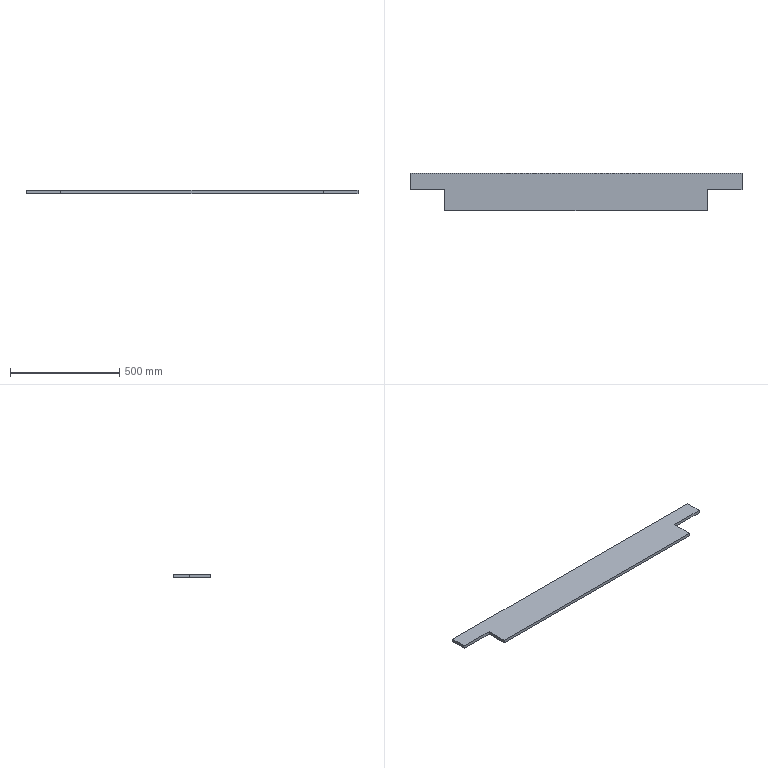Part | SolidWorks | features BaseBody 1 | 1 solid | 10 faces | box 1520 x 172 x 14 mm | volume 3225600 mm3 | plane 10
STEP:
#1=CARTESIAN_POINT('',(-600.,-84.5,14.));
#2=VERTEX_POINT('',#1);
#3=CARTESIAN_POINT('',(-600.,12.5,14.));
#4=VERTEX_POINT('',#3);
#5=CARTESIAN_POINT('',(-600.,12.5,14.));
#6=DIRECTION('',(0.,1.,0.));
#7=VECTOR('',#6,1000.);
#8=LINE('',#5,#7);
#9=EDGE_CURVE('',#2,#4,#8,.T.);
#10=ORIENTED_EDGE('',*,*,#9,.F.);
#11=CARTESIAN_POINT('',(600.,-84.5,14.));
#12=VERTEX_POINT('',#11);
#13=CARTESIAN_POINT('',(-600.,-84.5,14.));
#14=DIRECTION('',(-1.,0.,0.));
#15=VECTOR('',#14,1000.);
#16=LINE('',#13,#15);
#17=EDGE_CURVE('',#12,#2,#16,.T.);
#18=ORIENTED_EDGE('',*,*,#17,.F.);
#19=CARTESIAN_POINT('',(600.,12.5,14.));
#20=VERTEX_POINT('',#19);
#21=CARTESIAN_POINT('',(600.,12.5,14.));
#22=DIRECTION('',(0.,-1.,0.));
#23=VECTOR('',#22,1000.);
#24=LINE('',#21,#23);
#25=EDGE_CURVE('',#20,#12,#24,.T.);
#26=ORIENTED_EDGE('',*,*,#25,.F.);
#27=CARTESIAN_POINT('',(760.,12.5,14.));
#28=VERTEX_POINT('',#27);
#29=CARTESIAN_POINT('',(760.,12.5,14.));
#30=DIRECTION('',(-1.,0.,0.));
#31=VECTOR('',#30,1000.);
#32=LINE('',#29,#31);
#33=EDGE_CURVE('',#28,#20,#32,.T.);
#34=ORIENTED_EDGE('',*,*,#33,.F.);
#35=CARTESIAN_POINT('',(760.,87.5,14.));
#36=VERTEX_POINT('',#35);
#37=CARTESIAN_POINT('',(760.,87.5,14.));
#38=DIRECTION('',(0.,1.,0.));
#39=VECTOR('',#38,1000.);
#40=LINE('',#37,#39);
#41=EDGE_CURVE('',#28,#36,#40,.T.);
#42=ORIENTED_EDGE('',*,*,#41,.T.);
#43=CARTESIAN_POINT('',(-760.,87.5,14.));
#44=VERTEX_POINT('',#43);
#45=CARTESIAN_POINT('',(-760.,87.5,14.));
#46=DIRECTION('',(-1.,0.,0.));
#47=VECTOR('',#46,1000.);
#48=LINE('',#45,#47);
#49=EDGE_CURVE('',#36,#44,#48,.T.);
#50=ORIENTED_EDGE('',*,*,#49,.T.);
#51=CARTESIAN_POINT('',(-760.,12.5,14.));
#52=VERTEX_POINT('',#51);
#53=CARTESIAN_POINT('',(-760.,87.5,14.));
#54=DIRECTION('',(0.,-1.,0.));
#55=VECTOR('',#54,1000.);
#56=LINE('',#53,#55);
#57=EDGE_CURVE('',#44,#52,#56,.T.);
#58=ORIENTED_EDGE('',*,*,#57,.T.);
#59=CARTESIAN_POINT('',(-760.,12.5,14.));
#60=DIRECTION('',(-1.,0.,0.));
#61=VECTOR('',#60,1000.);
#62=LINE('',#59,#61);
#63=EDGE_CURVE('',#4,#52,#62,.T.);
#64=ORIENTED_EDGE('',*,*,#63,.F.);
#65=EDGE_LOOP('',(#10,#18,#26,#34,#42,#50,#58,#64));
#66=FACE_OUTER_BOUND('',#65,.T.);
#67=CARTESIAN_POINT('',(0.,0.,14.));
#68=DIRECTION('',(0.,0.,1.));
#69=DIRECTION('',(1.,0.,0.));
#70=AXIS2_PLACEMENT_3D('',#67,#68,#69);
#71=PLANE('',#70);
#72=ADVANCED_FACE('',(#66),#71,.T.);
#73=CARTESIAN_POINT('',(-600.,-84.5,0.));
#74=VERTEX_POINT('',#73);
#75=CARTESIAN_POINT('',(600.,-84.5,0.));
#76=VERTEX_POINT('',#75);
#77=CARTESIAN_POINT('',(0.,-84.5,0.));
#78=DIRECTION('',(1.,0.,0.));
#79=VECTOR('',#78,1000.);
#80=LINE('',#77,#79);
#81=EDGE_CURVE('',#74,#76,#80,.T.);
#82=ORIENTED_EDGE('',*,*,#81,.F.);
#83=CARTESIAN_POINT('',(-600.,12.5,0.));
#84=VERTEX_POINT('',#83);
#85=CARTESIAN_POINT('',(-600.,12.5,0.));
#86=DIRECTION('',(0.,1.,0.));
#87=VECTOR('',#86,1000.);
#88=LINE('',#85,#87);
#89=EDGE_CURVE('',#74,#84,#88,.T.);
#90=ORIENTED_EDGE('',*,*,#89,.T.);
#91=CARTESIAN_POINT('',(-760.,12.5,0.));
#92=VERTEX_POINT('',#91);
#93=CARTESIAN_POINT('',(-760.,12.5,0.));
#94=DIRECTION('',(-1.,0.,0.));
#95=VECTOR('',#94,1000.);
#96=LINE('',#93,#95);
#97=EDGE_CURVE('',#84,#92,#96,.T.);
#98=ORIENTED_EDGE('',*,*,#97,.T.);
#99=CARTESIAN_POINT('',(-760.,87.5,0.));
#100=VERTEX_POINT('',#99);
#101=CARTESIAN_POINT('',(-760.,87.5,0.));
#102=DIRECTION('',(0.,-1.,0.));
#103=VECTOR('',#102,1000.);
#104=LINE('',#101,#103);
#105=EDGE_CURVE('',#100,#92,#104,.T.);
#106=ORIENTED_EDGE('',*,*,#105,.F.);
#107=CARTESIAN_POINT('',(760.,87.5,0.));
#108=VERTEX_POINT('',#107);
#109=CARTESIAN_POINT('',(-760.,87.5,0.));
#110=DIRECTION('',(-1.,0.,0.));
#111=VECTOR('',#110,1000.);
#112=LINE('',#109,#111);
#113=EDGE_CURVE('',#108,#100,#112,.T.);
#114=ORIENTED_EDGE('',*,*,#113,.F.);
#115=CARTESIAN_POINT('',(760.,12.5,0.));
#116=VERTEX_POINT('',#115);
#117=CARTESIAN_POINT('',(760.,87.5,0.));
#118=DIRECTION('',(0.,1.,0.));
#119=VECTOR('',#118,1000.);
#120=LINE('',#117,#119);
#121=EDGE_CURVE('',#116,#108,#120,.T.);
#122=ORIENTED_EDGE('',*,*,#121,.F.);
#123=CARTESIAN_POINT('',(600.,12.5,0.));
#124=VERTEX_POINT('',#123);
#125=CARTESIAN_POINT('',(760.,12.5,0.));
#126=DIRECTION('',(-1.,0.,0.));
#127=VECTOR('',#126,1000.);
#128=LINE('',#125,#127);
#129=EDGE_CURVE('',#116,#124,#128,.T.);
#130=ORIENTED_EDGE('',*,*,#129,.T.);
#131=CARTESIAN_POINT('',(600.,12.5,0.));
#132=DIRECTION('',(0.,-1.,0.));
#133=VECTOR('',#132,1000.);
#134=LINE('',#131,#133);
#135=EDGE_CURVE('',#124,#76,#134,.T.);
#136=ORIENTED_EDGE('',*,*,#135,.T.);
#137=EDGE_LOOP('',(#82,#90,#98,#106,#114,#122,#130,#136));
#138=FACE_OUTER_BOUND('',#137,.T.);
#139=CARTESIAN_POINT('',(0.,0.,0.));
#140=DIRECTION('',(0.,0.,1.));
#141=DIRECTION('',(1.,0.,0.));
#142=AXIS2_PLACEMENT_3D('',#139,#140,#141);
#143=PLANE('',#142);
#144=ADVANCED_FACE('',(#138),#143,.F.);
#145=CARTESIAN_POINT('',(600.,-84.5,14.));
#146=DIRECTION('',(0.,0.,1.));
#147=VECTOR('',#146,1000.);
#148=LINE('',#145,#147);
#149=EDGE_CURVE('',#76,#12,#148,.T.);
#150=ORIENTED_EDGE('',*,*,#149,.F.);
#151=ORIENTED_EDGE('',*,*,#135,.F.);
#152=CARTESIAN_POINT('',(600.,12.5,0.));
#153=DIRECTION('',(0.,0.,1.));
#154=VECTOR('',#153,1000.);
#155=LINE('',#152,#154);
#156=EDGE_CURVE('',#124,#20,#155,.T.);
#157=ORIENTED_EDGE('',*,*,#156,.T.);
#158=ORIENTED_EDGE('',*,*,#25,.T.);
#159=EDGE_LOOP('',(#150,#151,#157,#158));
#160=FACE_OUTER_BOUND('',#159,.T.);
#161=CARTESIAN_POINT('',(600.,12.5,0.));
#162=DIRECTION('',(-1.,0.,0.));
#163=DIRECTION('',(0.,0.,1.));
#164=AXIS2_PLACEMENT_3D('',#161,#162,#163);
#165=PLANE('',#164);
#166=ADVANCED_FACE('',(#160),#165,.F.);
#167=CARTESIAN_POINT('',(-600.,-84.5,14.));
#168=DIRECTION('',(0.,0.,-1.));
#169=VECTOR('',#168,1000.);
#170=LINE('',#167,#169);
#171=EDGE_CURVE('',#2,#74,#170,.T.);
#172=ORIENTED_EDGE('',*,*,#171,.F.);
#173=ORIENTED_EDGE('',*,*,#9,.T.);
#174=CARTESIAN_POINT('',(-600.,12.5,0.));
#175=DIRECTION('',(0.,0.,1.));
#176=VECTOR('',#175,1000.);
#177=LINE('',#174,#176);
#178=EDGE_CURVE('',#84,#4,#177,.T.);
#179=ORIENTED_EDGE('',*,*,#178,.F.);
#180=ORIENTED_EDGE('',*,*,#89,.F.);
#181=EDGE_LOOP('',(#172,#173,#179,#180));
#182=FACE_OUTER_BOUND('',#181,.T.);
#183=CARTESIAN_POINT('',(-600.,12.5,0.));
#184=DIRECTION('',(1.,0.,0.));
#185=DIRECTION('',(0.,0.,-1.));
#186=AXIS2_PLACEMENT_3D('',#183,#184,#185);
#187=PLANE('',#186);
#188=ADVANCED_FACE('',(#182),#187,.F.);
#189=ORIENTED_EDGE('',*,*,#41,.F.);
#190=CARTESIAN_POINT('',(760.,12.5,0.));
#191=DIRECTION('',(0.,0.,1.));
#192=VECTOR('',#191,1000.);
#193=LINE('',#190,#192);
#194=EDGE_CURVE('',#116,#28,#193,.T.);
#195=ORIENTED_EDGE('',*,*,#194,.F.);
#196=ORIENTED_EDGE('',*,*,#121,.T.);
#197=CARTESIAN_POINT('',(760.,87.5,14.));
#198=DIRECTION('',(0.,0.,-1.));
#199=VECTOR('',#198,1000.);
#200=LINE('',#197,#199);
#201=EDGE_CURVE('',#36,#108,#200,.T.);
#202=ORIENTED_EDGE('',*,*,#201,.F.);
#203=EDGE_LOOP('',(#189,#195,#196,#202));
#204=FACE_OUTER_BOUND('',#203,.T.);
#205=CARTESIAN_POINT('',(760.,87.5,14.));
#206=DIRECTION('',(-1.,0.,0.));
#207=DIRECTION('',(0.,0.,1.));
#208=AXIS2_PLACEMENT_3D('',#205,#206,#207);
#209=PLANE('',#208);
#210=ADVANCED_FACE('',(#204),#209,.F.);
#211=ORIENTED_EDGE('',*,*,#113,.T.);
#212=CARTESIAN_POINT('',(-760.,87.5,14.));
#213=DIRECTION('',(0.,0.,-1.));
#214=VECTOR('',#213,1000.);
#215=LINE('',#212,#214);
#216=EDGE_CURVE('',#44,#100,#215,.T.);
#217=ORIENTED_EDGE('',*,*,#216,.F.);
#218=ORIENTED_EDGE('',*,*,#49,.F.);
#219=ORIENTED_EDGE('',*,*,#201,.T.);
#220=EDGE_LOOP('',(#211,#217,#218,#219));
#221=FACE_OUTER_BOUND('',#220,.T.);
#222=CARTESIAN_POINT('',(-760.,87.5,14.));
#223=DIRECTION('',(0.,-1.,0.));
#224=DIRECTION('',(0.,0.,-1.));
#225=AXIS2_PLACEMENT_3D('',#222,#223,#224);
#226=PLANE('',#225);
#227=ADVANCED_FACE('',(#221),#226,.F.);
#228=ORIENTED_EDGE('',*,*,#105,.T.);
#229=CARTESIAN_POINT('',(-760.,12.5,0.));
#230=DIRECTION('',(0.,0.,1.));
#231=VECTOR('',#230,1000.);
#232=LINE('',#229,#231);
#233=EDGE_CURVE('',#92,#52,#232,.T.);
#234=ORIENTED_EDGE('',*,*,#233,.T.);
#235=ORIENTED_EDGE('',*,*,#57,.F.);
#236=ORIENTED_EDGE('',*,*,#216,.T.);
#237=EDGE_LOOP('',(#228,#234,#235,#236));
#238=FACE_OUTER_BOUND('',#237,.T.);
#239=CARTESIAN_POINT('',(-760.,87.5,14.));
#240=DIRECTION('',(1.,0.,0.));
#241=DIRECTION('',(0.,0.,-1.));
#242=AXIS2_PLACEMENT_3D('',#239,#240,#241);
#243=PLANE('',#242);
#244=ADVANCED_FACE('',(#238),#243,.F.);
#245=ORIENTED_EDGE('',*,*,#33,.T.);
#246=ORIENTED_EDGE('',*,*,#156,.F.);
#247=ORIENTED_EDGE('',*,*,#129,.F.);
#248=ORIENTED_EDGE('',*,*,#194,.T.);
#249=EDGE_LOOP('',(#245,#246,#247,#248));
#250=FACE_OUTER_BOUND('',#249,.T.);
#251=CARTESIAN_POINT('',(760.,12.5,0.));
#252=DIRECTION('',(0.,1.,0.));
#253=DIRECTION('',(0.,0.,1.));
#254=AXIS2_PLACEMENT_3D('',#251,#252,#253);
#255=PLANE('',#254);
#256=ADVANCED_FACE('',(#250),#255,.F.);
#257=ORIENTED_EDGE('',*,*,#63,.T.);
#258=ORIENTED_EDGE('',*,*,#233,.F.);
#259=ORIENTED_EDGE('',*,*,#97,.F.);
#260=ORIENTED_EDGE('',*,*,#178,.T.);
#261=EDGE_LOOP('',(#257,#258,#259,#260));
#262=FACE_OUTER_BOUND('',#261,.T.);
#263=CARTESIAN_POINT('',(-760.,12.5,0.));
#264=DIRECTION('',(0.,1.,0.));
#265=DIRECTION('',(0.,0.,1.));
#266=AXIS2_PLACEMENT_3D('',#263,#264,#265);
#267=PLANE('',#266);
#268=ADVANCED_FACE('',(#262),#267,.F.);
#269=ORIENTED_EDGE('',*,*,#81,.T.);
#270=ORIENTED_EDGE('',*,*,#149,.T.);
#271=ORIENTED_EDGE('',*,*,#17,.T.);
#272=ORIENTED_EDGE('',*,*,#171,.T.);
#273=EDGE_LOOP('',(#269,#270,#271,#272));
#274=FACE_OUTER_BOUND('',#273,.T.);
#275=CARTESIAN_POINT('',(0.,-84.5,-56.));
#276=DIRECTION('',(0.,-1.,0.));
#277=DIRECTION('',(0.,0.,-1.));
#278=AXIS2_PLACEMENT_3D('',#275,#276,#277);
#279=PLANE('',#278);
#280=ADVANCED_FACE('',(#274),#279,.T.);
#281=CLOSED_SHELL('',(#72,#144,#166,#188,#210,#227,#244,#256,#268,#280));
#282=MANIFOLD_SOLID_BREP('',#281);
#283=CARTESIAN_POINT('',(0.,0.,0.));
#284=DIRECTION('',(0.,0.,1.));
#285=DIRECTION('',(1.,0.,0.));
#286=AXIS2_PLACEMENT_3D('',#283,#284,#285);
#287=(LENGTH_UNIT()NAMED_UNIT(*)SI_UNIT(.MILLI.,.METRE.));
#288=UNCERTAINTY_MEASURE_WITH_UNIT(LENGTH_MEASURE(0.00001),#287,'','');
#289=(NAMED_UNIT(*)PLANE_ANGLE_UNIT()SI_UNIT($,.RADIAN.));
#290=(NAMED_UNIT(*)SI_UNIT($,.STERADIAN.)SOLID_ANGLE_UNIT());
#291=(GEOMETRIC_REPRESENTATION_CONTEXT(3)GLOBAL_UNCERTAINTY_ASSIGNED_CONTEXT((#288))GLOBAL_UNIT_ASSIGNED_CONTEXT((#287,#289,#290))REPRESENTATION_CONTEXT('',''));
#292=ADVANCED_BREP_SHAPE_REPRESENTATION('',(#282,#286),#291);